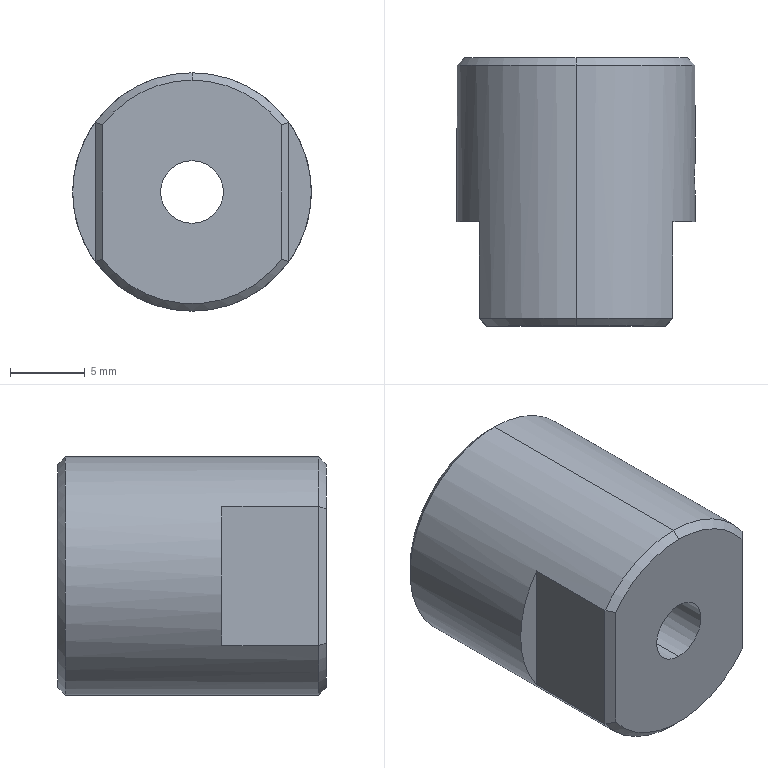Part | STEP file | OP10-128_seal head M6 | 1 solid | 27 faces | box 16 x 18 x 16 mm | volume 2771 mm3 | cylinder 10 | plane 10 | cone 7 | commonest cylinder face diameters 2 x2 4.2 x2 10.1 x2 11.5 x2 16 x2